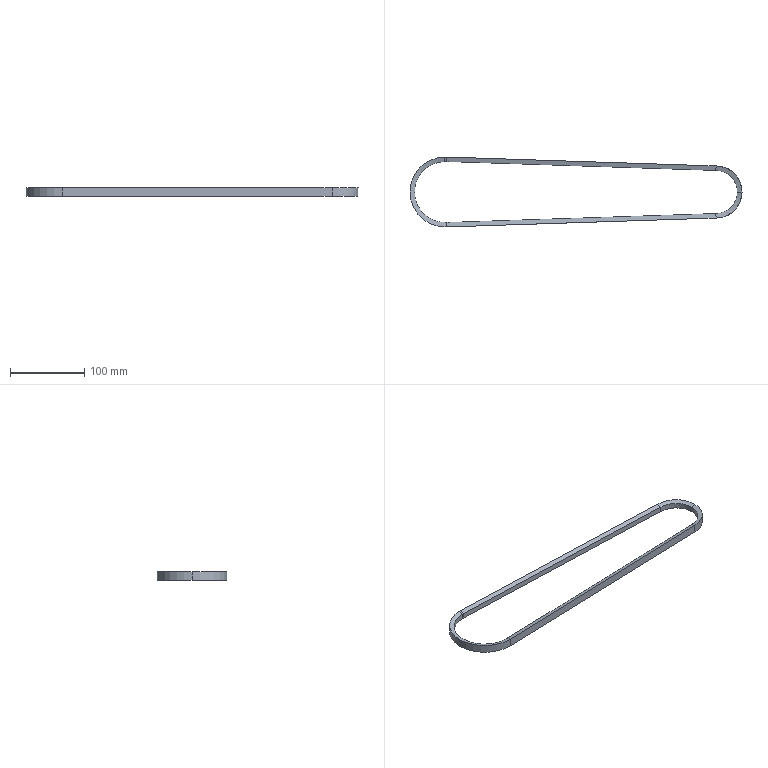Part | STEP file | Short V-belt | 1 solid | 24 faces | box 446 x 94 x 11 mm | volume 53257 mm3 | cone 8 | cylinder 8 | plane 8 | commonest cylinder face diameters 82 x3 94 x3 58 x1 70 x1
STEP:
#1=CARTESIAN_POINT('',(364.,29.,3.666));
#2=VERTEX_POINT('',#1);
#3=CARTESIAN_POINT('',(393.,0.,3.666));
#4=VERTEX_POINT('',#3);
#5=CARTESIAN_POINT('',(364.,0.,3.666));
#6=DIRECTION('',(0.,0.,-1.));
#7=DIRECTION('',(0.,1.,0.));
#8=AXIS2_PLACEMENT_3D('',#5,#6,#7);
#9=CIRCLE('',#8,29.);
#10=EDGE_CURVE('',#2,#4,#9,.T.);
#11=ORIENTED_EDGE('',*,*,#10,.T.);
#12=CARTESIAN_POINT('',(399.,0.,5.5));
#13=VERTEX_POINT('',#12);
#14=CARTESIAN_POINT('',(399.,0.,5.5));
#15=DIRECTION('',(0.9563,0.,0.2924));
#16=VECTOR('',#15,1000.);
#17=LINE('',#14,#16);
#18=EDGE_CURVE('',#4,#13,#17,.T.);
#19=ORIENTED_EDGE('',*,*,#18,.T.);
#20=CARTESIAN_POINT('',(364.104,35.,5.5));
#21=VERTEX_POINT('',#20);
#22=CARTESIAN_POINT('',(364.,0.,5.5));
#23=DIRECTION('',(0.,0.,-1.));
#24=DIRECTION('',(0.,1.,0.));
#25=AXIS2_PLACEMENT_3D('',#22,#23,#24);
#26=CIRCLE('',#25,35.);
#27=EDGE_CURVE('',#21,#13,#26,.T.);
#28=ORIENTED_EDGE('',*,*,#27,.F.);
#29=CARTESIAN_POINT('',(364.,29.,3.666));
#30=CARTESIAN_POINT('',(364.033,31.,4.277));
#31=CARTESIAN_POINT('',(364.068,33.,4.889));
#32=CARTESIAN_POINT('',(364.104,35.,5.5));
#33=B_SPLINE_CURVE_WITH_KNOTS('',3,(#29,#30,#31,#32),.UNSPECIFIED.,.F.,.F.,(4,4),(0.000000209,0.006275),.UNSPECIFIED.);
#34=EDGE_CURVE('',#2,#21,#33,.T.);
#35=ORIENTED_EDGE('',*,*,#34,.F.);
#36=EDGE_LOOP('',(#11,#19,#28,#35));
#37=FACE_OUTER_BOUND('',#36,.T.);
#38=CARTESIAN_POINT('',(364.,0.,5.5));
#39=DIRECTION('',(0.,0.,1.));
#40=DIRECTION('',(1.,0.,0.));
#41=AXIS2_PLACEMENT_3D('',#38,#39,#40);
#42=CONICAL_SURFACE('',#41,35.,1.274);
#43=ADVANCED_FACE('',(#37),#42,.F.);
#44=CARTESIAN_POINT('',(1.551,-46.974,5.5));
#45=VERTEX_POINT('',#44);
#46=CARTESIAN_POINT('',(-47.,0.,5.5));
#47=VERTEX_POINT('',#46);
#48=CARTESIAN_POINT('',(0.,0.,5.5));
#49=DIRECTION('',(0.,0.,-1.));
#50=DIRECTION('',(0.03301,-0.9995,0.));
#51=AXIS2_PLACEMENT_3D('',#48,#49,#50);
#52=CIRCLE('',#51,47.);
#53=EDGE_CURVE('',#45,#47,#52,.T.);
#54=ORIENTED_EDGE('',*,*,#53,.T.);
#55=CARTESIAN_POINT('',(-47.,0.,-5.5));
#56=VERTEX_POINT('',#55);
#57=CARTESIAN_POINT('',(-47.,0.,0.));
#58=DIRECTION('',(0.,0.,-1.));
#59=VECTOR('',#58,1000.);
#60=LINE('',#57,#59);
#61=EDGE_CURVE('',#47,#56,#60,.T.);
#62=ORIENTED_EDGE('',*,*,#61,.T.);
#63=CARTESIAN_POINT('',(1.551,-46.974,-5.5));
#64=VERTEX_POINT('',#63);
#65=CARTESIAN_POINT('',(0.,0.,-5.5));
#66=DIRECTION('',(0.,0.,-1.));
#67=DIRECTION('',(0.03301,-0.9995,0.));
#68=AXIS2_PLACEMENT_3D('',#65,#66,#67);
#69=CIRCLE('',#68,47.);
#70=EDGE_CURVE('',#64,#56,#69,.T.);
#71=ORIENTED_EDGE('',*,*,#70,.F.);
#72=CARTESIAN_POINT('',(1.551,-46.974,5.5));
#73=DIRECTION('',(0.,0.,1.));
#74=VECTOR('',#73,1000.);
#75=LINE('',#72,#74);
#76=EDGE_CURVE('',#64,#45,#75,.T.);
#77=ORIENTED_EDGE('',*,*,#76,.T.);
#78=EDGE_LOOP('',(#54,#62,#71,#77));
#79=FACE_OUTER_BOUND('',#78,.T.);
#80=CARTESIAN_POINT('',(0.,0.,0.));
#81=DIRECTION('',(0.,0.,-1.));
#82=DIRECTION('',(-1.,0.,0.));
#83=AXIS2_PLACEMENT_3D('',#80,#81,#82);
#84=CYLINDRICAL_SURFACE('',#83,47.);
#85=ADVANCED_FACE('',(#79),#84,.T.);
#86=CARTESIAN_POINT('',(-41.,0.,-3.666));
#87=VERTEX_POINT('',#86);
#88=CARTESIAN_POINT('',(0.,41.,-3.666));
#89=VERTEX_POINT('',#88);
#90=CARTESIAN_POINT('',(0.,0.,-3.666));
#91=DIRECTION('',(0.,0.,-1.));
#92=DIRECTION('',(0.03301,-0.9995,0.));
#93=AXIS2_PLACEMENT_3D('',#90,#91,#92);
#94=CIRCLE('',#93,41.);
#95=EDGE_CURVE('',#87,#89,#94,.T.);
#96=ORIENTED_EDGE('',*,*,#95,.F.);
#97=CARTESIAN_POINT('',(-41.,0.,-3.666));
#98=DIRECTION('',(-0.9563,0.,-0.2924));
#99=VECTOR('',#98,1000.);
#100=LINE('',#97,#99);
#101=EDGE_CURVE('',#87,#56,#100,.T.);
#102=ORIENTED_EDGE('',*,*,#101,.T.);
#103=CARTESIAN_POINT('',(0.,47.,-5.5));
#104=VERTEX_POINT('',#103);
#105=CARTESIAN_POINT('',(0.,0.,-5.5));
#106=DIRECTION('',(0.,0.,-1.));
#107=DIRECTION('',(0.03301,-0.9995,0.));
#108=AXIS2_PLACEMENT_3D('',#105,#106,#107);
#109=CIRCLE('',#108,47.);
#110=EDGE_CURVE('',#56,#104,#109,.T.);
#111=ORIENTED_EDGE('',*,*,#110,.T.);
#112=CARTESIAN_POINT('',(0.,47.,-5.5));
#113=DIRECTION('',(0.,0.9563,-0.2924));
#114=VECTOR('',#113,1000.);
#115=LINE('',#112,#114);
#116=EDGE_CURVE('',#89,#104,#115,.T.);
#117=ORIENTED_EDGE('',*,*,#116,.F.);
#118=EDGE_LOOP('',(#96,#102,#111,#117));
#119=FACE_OUTER_BOUND('',#118,.T.);
#120=CARTESIAN_POINT('',(0.,0.,-3.666));
#121=DIRECTION('',(0.,0.,-1.));
#122=DIRECTION('',(-1.,0.,0.));
#123=AXIS2_PLACEMENT_3D('',#120,#121,#122);
#124=CONICAL_SURFACE('',#123,41.,1.274);
#125=ADVANCED_FACE('',(#119),#124,.F.);
#126=CARTESIAN_POINT('',(-41.,0.,3.666));
#127=VERTEX_POINT('',#126);
#128=CARTESIAN_POINT('',(0.,41.,3.666));
#129=VERTEX_POINT('',#128);
#130=CARTESIAN_POINT('',(0.,0.,3.666));
#131=DIRECTION('',(0.,0.,-1.));
#132=DIRECTION('',(0.03301,-0.9995,0.));
#133=AXIS2_PLACEMENT_3D('',#130,#131,#132);
#134=CIRCLE('',#133,41.);
#135=EDGE_CURVE('',#127,#129,#134,.T.);
#136=ORIENTED_EDGE('',*,*,#135,.F.);
#137=CARTESIAN_POINT('',(-41.,0.,0.));
#138=DIRECTION('',(0.,0.,-1.));
#139=VECTOR('',#138,1000.);
#140=LINE('',#137,#139);
#141=EDGE_CURVE('',#127,#87,#140,.T.);
#142=ORIENTED_EDGE('',*,*,#141,.T.);
#143=ORIENTED_EDGE('',*,*,#95,.T.);
#144=CARTESIAN_POINT('',(0.,41.,-3.666));
#145=DIRECTION('',(0.,0.,-1.));
#146=VECTOR('',#145,1000.);
#147=LINE('',#144,#146);
#148=EDGE_CURVE('',#129,#89,#147,.T.);
#149=ORIENTED_EDGE('',*,*,#148,.F.);
#150=EDGE_LOOP('',(#136,#142,#143,#149));
#151=FACE_OUTER_BOUND('',#150,.T.);
#152=CARTESIAN_POINT('',(0.,0.,0.));
#153=DIRECTION('',(0.,0.,-1.));
#154=DIRECTION('',(-1.,0.,0.));
#155=AXIS2_PLACEMENT_3D('',#152,#153,#154);
#156=CYLINDRICAL_SURFACE('',#155,41.);
#157=ADVANCED_FACE('',(#151),#156,.F.);
#158=ORIENTED_EDGE('',*,*,#18,.F.);
#159=CARTESIAN_POINT('',(364.,-29.,3.666));
#160=VERTEX_POINT('',#159);
#161=CARTESIAN_POINT('',(364.,0.,3.666));
#162=DIRECTION('',(0.,0.,-1.));
#163=DIRECTION('',(0.,1.,0.));
#164=AXIS2_PLACEMENT_3D('',#161,#162,#163);
#165=CIRCLE('',#164,29.);
#166=EDGE_CURVE('',#4,#160,#165,.T.);
#167=ORIENTED_EDGE('',*,*,#166,.T.);
#168=CARTESIAN_POINT('',(364.104,-35.,5.5));
#169=VERTEX_POINT('',#168);
#170=CARTESIAN_POINT('',(364.,-29.,3.666));
#171=CARTESIAN_POINT('',(364.033,-31.,4.277));
#172=CARTESIAN_POINT('',(364.068,-33.,4.889));
#173=CARTESIAN_POINT('',(364.104,-35.,5.5));
#174=B_SPLINE_CURVE_WITH_KNOTS('',3,(#170,#171,#172,#173),.UNSPECIFIED.,.F.,.F.,(4,4),(0.000000209,0.006275),.UNSPECIFIED.);
#175=EDGE_CURVE('',#160,#169,#174,.T.);
#176=ORIENTED_EDGE('',*,*,#175,.T.);
#177=CARTESIAN_POINT('',(364.,0.,5.5));
#178=DIRECTION('',(0.,0.,-1.));
#179=DIRECTION('',(0.,1.,0.));
#180=AXIS2_PLACEMENT_3D('',#177,#178,#179);
#181=CIRCLE('',#180,35.);
#182=EDGE_CURVE('',#13,#169,#181,.T.);
#183=ORIENTED_EDGE('',*,*,#182,.F.);
#184=EDGE_LOOP('',(#158,#167,#176,#183));
#185=FACE_OUTER_BOUND('',#184,.T.);
#186=CARTESIAN_POINT('',(364.,0.,5.5));
#187=DIRECTION('',(0.,0.,1.));
#188=DIRECTION('',(1.,0.,0.));
#189=AXIS2_PLACEMENT_3D('',#186,#187,#188);
#190=CONICAL_SURFACE('',#189,35.,1.274);
#191=ADVANCED_FACE('',(#185),#190,.F.);
#192=CARTESIAN_POINT('',(364.104,35.,-5.5));
#193=VERTEX_POINT('',#192);
#194=CARTESIAN_POINT('',(364.,29.,-3.666));
#195=VERTEX_POINT('',#194);
#196=CARTESIAN_POINT('',(364.104,35.,-5.5));
#197=CARTESIAN_POINT('',(364.068,33.,-4.889));
#198=CARTESIAN_POINT('',(364.033,31.,-4.277));
#199=CARTESIAN_POINT('',(364.,29.,-3.666));
#200=B_SPLINE_CURVE_WITH_KNOTS('',3,(#196,#197,#198,#199),.UNSPECIFIED.,.F.,.F.,(4,4),(0.00000037,0.006275),.UNSPECIFIED.);
#201=EDGE_CURVE('',#193,#195,#200,.T.);
#202=ORIENTED_EDGE('',*,*,#201,.F.);
#203=CARTESIAN_POINT('',(364.104,-35.,-5.5));
#204=VERTEX_POINT('',#203);
#205=CARTESIAN_POINT('',(364.,0.,-5.5));
#206=DIRECTION('',(0.,0.,-1.));
#207=DIRECTION('',(0.,1.,0.));
#208=AXIS2_PLACEMENT_3D('',#205,#206,#207);
#209=CIRCLE('',#208,35.);
#210=EDGE_CURVE('',#193,#204,#209,.T.);
#211=ORIENTED_EDGE('',*,*,#210,.T.);
#212=CARTESIAN_POINT('',(364.,-29.,-3.666));
#213=VERTEX_POINT('',#212);
#214=CARTESIAN_POINT('',(364.104,-35.,-5.5));
#215=CARTESIAN_POINT('',(364.068,-33.,-4.889));
#216=CARTESIAN_POINT('',(364.033,-31.,-4.277));
#217=CARTESIAN_POINT('',(364.,-29.,-3.666));
#218=B_SPLINE_CURVE_WITH_KNOTS('',3,(#214,#215,#216,#217),.UNSPECIFIED.,.F.,.F.,(4,4),(0.00000037,0.006275),.UNSPECIFIED.);
#219=EDGE_CURVE('',#204,#213,#218,.T.);
#220=ORIENTED_EDGE('',*,*,#219,.T.);
#221=CARTESIAN_POINT('',(364.,0.,-3.666));
#222=DIRECTION('',(0.,0.,-1.));
#223=DIRECTION('',(0.,1.,0.));
#224=AXIS2_PLACEMENT_3D('',#221,#222,#223);
#225=CIRCLE('',#224,29.);
#226=EDGE_CURVE('',#195,#213,#225,.T.);
#227=ORIENTED_EDGE('',*,*,#226,.F.);
#228=EDGE_LOOP('',(#202,#211,#220,#227));
#229=FACE_OUTER_BOUND('',#228,.T.);
#230=CARTESIAN_POINT('',(364.,0.,-3.666));
#231=DIRECTION('',(0.,0.,-1.));
#232=DIRECTION('',(-1.,0.,0.));
#233=AXIS2_PLACEMENT_3D('',#230,#231,#232);
#234=CONICAL_SURFACE('',#233,29.,1.274);
#235=ADVANCED_FACE('',(#229),#234,.F.);
#236=ORIENTED_EDGE('',*,*,#210,.F.);
#237=CARTESIAN_POINT('',(364.104,35.,0.));
#238=DIRECTION('',(0.,0.,1.));
#239=VECTOR('',#238,1000.);
#240=LINE('',#237,#239);
#241=EDGE_CURVE('',#193,#21,#240,.T.);
#242=ORIENTED_EDGE('',*,*,#241,.T.);
#243=ORIENTED_EDGE('',*,*,#27,.T.);
#244=ORIENTED_EDGE('',*,*,#182,.T.);
#245=CARTESIAN_POINT('',(364.104,-35.,0.));
#246=DIRECTION('',(0.,0.,1.));
#247=VECTOR('',#246,1000.);
#248=LINE('',#245,#247);
#249=EDGE_CURVE('',#204,#169,#248,.T.);
#250=ORIENTED_EDGE('',*,*,#249,.F.);
#251=EDGE_LOOP('',(#236,#242,#243,#244,#250));
#252=FACE_OUTER_BOUND('',#251,.T.);
#253=CARTESIAN_POINT('',(364.,0.,0.));
#254=DIRECTION('',(0.,0.,-1.));
#255=DIRECTION('',(-1.,0.,0.));
#256=AXIS2_PLACEMENT_3D('',#253,#254,#255);
#257=CYLINDRICAL_SURFACE('',#256,35.);
#258=ADVANCED_FACE('',(#252),#257,.T.);
#259=ORIENTED_EDGE('',*,*,#226,.T.);
#260=CARTESIAN_POINT('',(364.,-29.,-3.666));
#261=DIRECTION('',(0.,0.,-1.));
#262=VECTOR('',#261,1000.);
#263=LINE('',#260,#262);
#264=EDGE_CURVE('',#160,#213,#263,.T.);
#265=ORIENTED_EDGE('',*,*,#264,.F.);
#266=ORIENTED_EDGE('',*,*,#166,.F.);
#267=ORIENTED_EDGE('',*,*,#10,.F.);
#268=CARTESIAN_POINT('',(364.,29.,-3.666));
#269=DIRECTION('',(0.,0.,-1.));
#270=VECTOR('',#269,1000.);
#271=LINE('',#268,#270);
#272=EDGE_CURVE('',#2,#195,#271,.T.);
#273=ORIENTED_EDGE('',*,*,#272,.T.);
#274=EDGE_LOOP('',(#259,#265,#266,#267,#273));
#275=FACE_OUTER_BOUND('',#274,.T.);
#276=CARTESIAN_POINT('',(364.,0.,0.));
#277=DIRECTION('',(0.,0.,-1.));
#278=DIRECTION('',(-1.,0.,0.));
#279=AXIS2_PLACEMENT_3D('',#276,#277,#278);
#280=CYLINDRICAL_SURFACE('',#279,29.);
#281=ADVANCED_FACE('',(#275),#280,.F.);
#282=ORIENTED_EDGE('',*,*,#175,.F.);
#283=CARTESIAN_POINT('',(1.353,-40.978,3.666));
#284=VERTEX_POINT('',#283);
#285=CARTESIAN_POINT('',(364.,-29.,3.666));
#286=DIRECTION('',(-0.9995,-0.03301,0.));
#287=VECTOR('',#286,1000.);
#288=LINE('',#285,#287);
#289=EDGE_CURVE('',#160,#284,#288,.T.);
#290=ORIENTED_EDGE('',*,*,#289,.T.);
#291=CARTESIAN_POINT('',(1.551,-46.974,5.5));
#292=DIRECTION('',(-0.03157,0.9558,-0.2924));
#293=VECTOR('',#292,1000.);
#294=LINE('',#291,#293);
#295=EDGE_CURVE('',#45,#284,#294,.T.);
#296=ORIENTED_EDGE('',*,*,#295,.F.);
#297=CARTESIAN_POINT('',(364.198,-34.997,5.5));
#298=DIRECTION('',(-0.9995,-0.03301,0.));
#299=VECTOR('',#298,1000.);
#300=LINE('',#297,#299);
#301=EDGE_CURVE('',#169,#45,#300,.T.);
#302=ORIENTED_EDGE('',*,*,#301,.F.);
#303=EDGE_LOOP('',(#282,#290,#296,#302));
#304=FACE_OUTER_BOUND('',#303,.T.);
#305=CARTESIAN_POINT('',(364.198,-34.997,5.5));
#306=DIRECTION('',(-0.009651,0.2922,0.9563));
#307=DIRECTION('',(0.,-0.9563,0.2922));
#308=AXIS2_PLACEMENT_3D('',#305,#306,#307);
#309=PLANE('',#308);
#310=ADVANCED_FACE('',(#304),#309,.T.);
#311=ORIENTED_EDGE('',*,*,#219,.F.);
#312=CARTESIAN_POINT('',(364.198,-34.997,-5.5));
#313=DIRECTION('',(-0.9995,-0.03301,0.));
#314=VECTOR('',#313,1000.);
#315=LINE('',#312,#314);
#316=EDGE_CURVE('',#204,#64,#315,.T.);
#317=ORIENTED_EDGE('',*,*,#316,.T.);
#318=CARTESIAN_POINT('',(1.353,-40.978,-3.666));
#319=VERTEX_POINT('',#318);
#320=CARTESIAN_POINT('',(1.551,-46.974,-5.5));
#321=DIRECTION('',(0.03157,-0.9558,-0.2924));
#322=VECTOR('',#321,1000.);
#323=LINE('',#320,#322);
#324=EDGE_CURVE('',#319,#64,#323,.T.);
#325=ORIENTED_EDGE('',*,*,#324,.F.);
#326=CARTESIAN_POINT('',(364.,-29.,-3.666));
#327=DIRECTION('',(-0.9995,-0.03301,0.));
#328=VECTOR('',#327,1000.);
#329=LINE('',#326,#328);
#330=EDGE_CURVE('',#213,#319,#329,.T.);
#331=ORIENTED_EDGE('',*,*,#330,.F.);
#332=EDGE_LOOP('',(#311,#317,#325,#331));
#333=FACE_OUTER_BOUND('',#332,.T.);
#334=CARTESIAN_POINT('',(364.198,-34.997,-5.5));
#335=DIRECTION('',(-0.009651,0.2922,-0.9563));
#336=DIRECTION('',(0.,0.9563,0.2922));
#337=AXIS2_PLACEMENT_3D('',#334,#335,#336);
#338=PLANE('',#337);
#339=ADVANCED_FACE('',(#333),#338,.T.);
#340=ORIENTED_EDGE('',*,*,#330,.T.);
#341=CARTESIAN_POINT('',(1.353,-40.978,-3.666));
#342=DIRECTION('',(0.,0.,-1.));
#343=VECTOR('',#342,1000.);
#344=LINE('',#341,#343);
#345=EDGE_CURVE('',#284,#319,#344,.T.);
#346=ORIENTED_EDGE('',*,*,#345,.F.);
#347=ORIENTED_EDGE('',*,*,#289,.F.);
#348=ORIENTED_EDGE('',*,*,#264,.T.);
#349=EDGE_LOOP('',(#340,#346,#347,#348));
#350=FACE_OUTER_BOUND('',#349,.T.);
#351=CARTESIAN_POINT('',(364.,-29.,-3.666));
#352=DIRECTION('',(-0.03301,0.9995,0.));
#353=DIRECTION('',(-0.9995,-0.03301,0.));
#354=AXIS2_PLACEMENT_3D('',#351,#352,#353);
#355=PLANE('',#354);
#356=ADVANCED_FACE('',(#350),#355,.T.);
#357=ORIENTED_EDGE('',*,*,#316,.F.);
#358=ORIENTED_EDGE('',*,*,#249,.T.);
#359=ORIENTED_EDGE('',*,*,#301,.T.);
#360=ORIENTED_EDGE('',*,*,#76,.F.);
#361=EDGE_LOOP('',(#357,#358,#359,#360));
#362=FACE_OUTER_BOUND('',#361,.T.);
#363=CARTESIAN_POINT('',(364.198,-34.997,5.5));
#364=DIRECTION('',(0.03301,-0.9995,0.));
#365=DIRECTION('',(0.9995,0.03301,0.));
#366=AXIS2_PLACEMENT_3D('',#363,#364,#365);
#367=PLANE('',#366);
#368=ADVANCED_FACE('',(#362),#367,.T.);
#369=CARTESIAN_POINT('',(1.353,40.978,3.666));
#370=VERTEX_POINT('',#369);
#371=CARTESIAN_POINT('',(1.353,40.978,3.666));
#372=DIRECTION('',(0.9995,-0.03301,0.));
#373=VECTOR('',#372,1000.);
#374=LINE('',#371,#373);
#375=EDGE_CURVE('',#370,#2,#374,.T.);
#376=ORIENTED_EDGE('',*,*,#375,.T.);
#377=ORIENTED_EDGE('',*,*,#34,.T.);
#378=CARTESIAN_POINT('',(1.551,46.974,5.5));
#379=VERTEX_POINT('',#378);
#380=CARTESIAN_POINT('',(1.551,46.974,5.5));
#381=DIRECTION('',(0.9995,-0.03301,0.));
#382=VECTOR('',#381,1000.);
#383=LINE('',#380,#382);
#384=EDGE_CURVE('',#379,#21,#383,.T.);
#385=ORIENTED_EDGE('',*,*,#384,.F.);
#386=CARTESIAN_POINT('',(1.551,46.974,5.5));
#387=DIRECTION('',(-0.03157,-0.9558,-0.2924));
#388=VECTOR('',#387,1000.);
#389=LINE('',#386,#388);
#390=EDGE_CURVE('',#379,#370,#389,.T.);
#391=ORIENTED_EDGE('',*,*,#390,.T.);
#392=EDGE_LOOP('',(#376,#377,#385,#391));
#393=FACE_OUTER_BOUND('',#392,.T.);
#394=CARTESIAN_POINT('',(1.551,46.974,5.5));
#395=DIRECTION('',(-0.009651,-0.2922,0.9563));
#396=DIRECTION('',(0.,-0.9563,-0.2922));
#397=AXIS2_PLACEMENT_3D('',#394,#395,#396);
#398=PLANE('',#397);
#399=ADVANCED_FACE('',(#393),#398,.T.);
#400=CARTESIAN_POINT('',(1.551,46.974,-5.5));
#401=VERTEX_POINT('',#400);
#402=CARTESIAN_POINT('',(1.551,46.974,-5.5));
#403=DIRECTION('',(0.9995,-0.03301,0.));
#404=VECTOR('',#403,1000.);
#405=LINE('',#402,#404);
#406=EDGE_CURVE('',#401,#193,#405,.T.);
#407=ORIENTED_EDGE('',*,*,#406,.T.);
#408=ORIENTED_EDGE('',*,*,#201,.T.);
#409=CARTESIAN_POINT('',(1.353,40.978,-3.666));
#410=VERTEX_POINT('',#409);
#411=CARTESIAN_POINT('',(1.353,40.978,-3.666));
#412=DIRECTION('',(0.9995,-0.03301,0.));
#413=VECTOR('',#412,1000.);
#414=LINE('',#411,#413);
#415=EDGE_CURVE('',#410,#195,#414,.T.);
#416=ORIENTED_EDGE('',*,*,#415,.F.);
#417=CARTESIAN_POINT('',(1.551,46.974,-5.5));
#418=DIRECTION('',(0.03157,0.9558,-0.2924));
#419=VECTOR('',#418,1000.);
#420=LINE('',#417,#419);
#421=EDGE_CURVE('',#410,#401,#420,.T.);
#422=ORIENTED_EDGE('',*,*,#421,.T.);
#423=EDGE_LOOP('',(#407,#408,#416,#422));
#424=FACE_OUTER_BOUND('',#423,.T.);
#425=CARTESIAN_POINT('',(1.551,46.974,-5.5));
#426=DIRECTION('',(-0.009651,-0.2922,-0.9563));
#427=DIRECTION('',(0.,0.9563,-0.2922));
#428=AXIS2_PLACEMENT_3D('',#425,#426,#427);
#429=PLANE('',#428);
#430=ADVANCED_FACE('',(#424),#429,.T.);
#431=ORIENTED_EDGE('',*,*,#241,.F.);
#432=ORIENTED_EDGE('',*,*,#406,.F.);
#433=CARTESIAN_POINT('',(1.551,46.974,5.5));
#434=DIRECTION('',(0.,0.,1.));
#435=VECTOR('',#434,1000.);
#436=LINE('',#433,#435);
#437=EDGE_CURVE('',#401,#379,#436,.T.);
#438=ORIENTED_EDGE('',*,*,#437,.T.);
#439=ORIENTED_EDGE('',*,*,#384,.T.);
#440=EDGE_LOOP('',(#431,#432,#438,#439));
#441=FACE_OUTER_BOUND('',#440,.T.);
#442=CARTESIAN_POINT('',(1.551,46.974,5.5));
#443=DIRECTION('',(0.03301,0.9995,0.));
#444=DIRECTION('',(-0.9995,0.03301,0.));
#445=AXIS2_PLACEMENT_3D('',#442,#443,#444);
#446=PLANE('',#445);
#447=ADVANCED_FACE('',(#441),#446,.T.);
#448=ORIENTED_EDGE('',*,*,#415,.T.);
#449=ORIENTED_EDGE('',*,*,#272,.F.);
#450=ORIENTED_EDGE('',*,*,#375,.F.);
#451=CARTESIAN_POINT('',(1.353,40.978,-3.666));
#452=DIRECTION('',(0.,0.,-1.));
#453=VECTOR('',#452,1000.);
#454=LINE('',#451,#453);
#455=EDGE_CURVE('',#370,#410,#454,.T.);
#456=ORIENTED_EDGE('',*,*,#455,.T.);
#457=EDGE_LOOP('',(#448,#449,#450,#456));
#458=FACE_OUTER_BOUND('',#457,.T.);
#459=CARTESIAN_POINT('',(1.353,40.978,-3.666));
#460=DIRECTION('',(-0.03301,-0.9995,0.));
#461=DIRECTION('',(0.9995,-0.03301,0.));
#462=AXIS2_PLACEMENT_3D('',#459,#460,#461);
#463=PLANE('',#462);
#464=ADVANCED_FACE('',(#458),#463,.T.);
#465=ORIENTED_EDGE('',*,*,#437,.F.);
#466=CARTESIAN_POINT('',(0.,0.,-5.5));
#467=DIRECTION('',(0.,0.,-1.));
#468=DIRECTION('',(0.,1.,0.));
#469=AXIS2_PLACEMENT_3D('',#466,#467,#468);
#470=CIRCLE('',#469,47.);
#471=EDGE_CURVE('',#104,#401,#470,.T.);
#472=ORIENTED_EDGE('',*,*,#471,.F.);
#473=CARTESIAN_POINT('',(0.,47.,5.5));
#474=VERTEX_POINT('',#473);
#475=CARTESIAN_POINT('',(0.,47.,5.5));
#476=DIRECTION('',(0.,0.,1.));
#477=VECTOR('',#476,1000.);
#478=LINE('',#475,#477);
#479=EDGE_CURVE('',#104,#474,#478,.T.);
#480=ORIENTED_EDGE('',*,*,#479,.T.);
#481=CARTESIAN_POINT('',(0.,0.,5.5));
#482=DIRECTION('',(0.,0.,-1.));
#483=DIRECTION('',(0.,1.,0.));
#484=AXIS2_PLACEMENT_3D('',#481,#482,#483);
#485=CIRCLE('',#484,47.);
#486=EDGE_CURVE('',#474,#379,#485,.T.);
#487=ORIENTED_EDGE('',*,*,#486,.T.);
#488=EDGE_LOOP('',(#465,#472,#480,#487));
#489=FACE_OUTER_BOUND('',#488,.T.);
#490=CARTESIAN_POINT('',(0.,0.,0.));
#491=DIRECTION('',(0.,0.,-1.));
#492=DIRECTION('',(-1.,0.,0.));
#493=AXIS2_PLACEMENT_3D('',#490,#491,#492);
#494=CYLINDRICAL_SURFACE('',#493,47.);
#495=ADVANCED_FACE('',(#489),#494,.T.);
#496=ORIENTED_EDGE('',*,*,#471,.T.);
#497=ORIENTED_EDGE('',*,*,#421,.F.);
#498=CARTESIAN_POINT('',(0.,0.,-3.666));
#499=DIRECTION('',(0.,0.,-1.));
#500=DIRECTION('',(0.,1.,0.));
#501=AXIS2_PLACEMENT_3D('',#498,#499,#500);
#502=CIRCLE('',#501,41.);
#503=EDGE_CURVE('',#89,#410,#502,.T.);
#504=ORIENTED_EDGE('',*,*,#503,.F.);
#505=ORIENTED_EDGE('',*,*,#116,.T.);
#506=EDGE_LOOP('',(#496,#497,#504,#505));
#507=FACE_OUTER_BOUND('',#506,.T.);
#508=CARTESIAN_POINT('',(0.,0.,-3.666));
#509=DIRECTION('',(0.,0.,-1.));
#510=DIRECTION('',(-1.,0.,0.));
#511=AXIS2_PLACEMENT_3D('',#508,#509,#510);
#512=CONICAL_SURFACE('',#511,41.,1.274);
#513=ADVANCED_FACE('',(#507),#512,.F.);
#514=ORIENTED_EDGE('',*,*,#503,.T.);
#515=ORIENTED_EDGE('',*,*,#455,.F.);
#516=CARTESIAN_POINT('',(0.,0.,3.666));
#517=DIRECTION('',(0.,0.,-1.));
#518=DIRECTION('',(0.,1.,0.));
#519=AXIS2_PLACEMENT_3D('',#516,#517,#518);
#520=CIRCLE('',#519,41.);
#521=EDGE_CURVE('',#129,#370,#520,.T.);
#522=ORIENTED_EDGE('',*,*,#521,.F.);
#523=ORIENTED_EDGE('',*,*,#148,.T.);
#524=EDGE_LOOP('',(#514,#515,#522,#523));
#525=FACE_OUTER_BOUND('',#524,.T.);
#526=CARTESIAN_POINT('',(0.,0.,0.));
#527=DIRECTION('',(0.,0.,-1.));
#528=DIRECTION('',(-1.,0.,0.));
#529=AXIS2_PLACEMENT_3D('',#526,#527,#528);
#530=CYLINDRICAL_SURFACE('',#529,41.);
#531=ADVANCED_FACE('',(#525),#530,.F.);
#532=ORIENTED_EDGE('',*,*,#521,.T.);
#533=ORIENTED_EDGE('',*,*,#390,.F.);
#534=ORIENTED_EDGE('',*,*,#486,.F.);
#535=CARTESIAN_POINT('',(0.,47.,5.5));
#536=DIRECTION('',(0.,-0.9563,-0.2924));
#537=VECTOR('',#536,1000.);
#538=LINE('',#535,#537);
#539=EDGE_CURVE('',#474,#129,#538,.T.);
#540=ORIENTED_EDGE('',*,*,#539,.T.);
#541=EDGE_LOOP('',(#532,#533,#534,#540));
#542=FACE_OUTER_BOUND('',#541,.T.);
#543=CARTESIAN_POINT('',(0.,0.,5.5));
#544=DIRECTION('',(0.,0.,1.));
#545=DIRECTION('',(1.,0.,0.));
#546=AXIS2_PLACEMENT_3D('',#543,#544,#545);
#547=CONICAL_SURFACE('',#546,47.,1.274);
#548=ADVANCED_FACE('',(#542),#547,.F.);
#549=ORIENTED_EDGE('',*,*,#61,.F.);
#550=CARTESIAN_POINT('',(0.,0.,5.5));
#551=DIRECTION('',(0.,0.,-1.));
#552=DIRECTION('',(0.03301,-0.9995,0.));
#553=AXIS2_PLACEMENT_3D('',#550,#551,#552);
#554=CIRCLE('',#553,47.);
#555=EDGE_CURVE('',#47,#474,#554,.T.);
#556=ORIENTED_EDGE('',*,*,#555,.T.);
#557=ORIENTED_EDGE('',*,*,#479,.F.);
#558=ORIENTED_EDGE('',*,*,#110,.F.);
#559=EDGE_LOOP('',(#549,#556,#557,#558));
#560=FACE_OUTER_BOUND('',#559,.T.);
#561=CARTESIAN_POINT('',(0.,0.,0.));
#562=DIRECTION('',(0.,0.,-1.));
#563=DIRECTION('',(-1.,0.,0.));
#564=AXIS2_PLACEMENT_3D('',#561,#562,#563);
#565=CYLINDRICAL_SURFACE('',#564,47.);
#566=ADVANCED_FACE('',(#560),#565,.T.);
#567=ORIENTED_EDGE('',*,*,#101,.F.);
#568=CARTESIAN_POINT('',(0.,0.,-3.666));
#569=DIRECTION('',(0.,0.,-1.));
#570=DIRECTION('',(0.03301,-0.9995,0.));
#571=AXIS2_PLACEMENT_3D('',#568,#569,#570);
#572=CIRCLE('',#571,41.);
#573=EDGE_CURVE('',#319,#87,#572,.T.);
#574=ORIENTED_EDGE('',*,*,#573,.F.);
#575=ORIENTED_EDGE('',*,*,#324,.T.);
#576=ORIENTED_EDGE('',*,*,#70,.T.);
#577=EDGE_LOOP('',(#567,#574,#575,#576));
#578=FACE_OUTER_BOUND('',#577,.T.);
#579=CARTESIAN_POINT('',(0.,0.,-3.666));
#580=DIRECTION('',(0.,0.,-1.));
#581=DIRECTION('',(-1.,0.,0.));
#582=AXIS2_PLACEMENT_3D('',#579,#580,#581);
#583=CONICAL_SURFACE('',#582,41.,1.274);
#584=ADVANCED_FACE('',(#578),#583,.F.);
#585=ORIENTED_EDGE('',*,*,#141,.F.);
#586=CARTESIAN_POINT('',(0.,0.,3.666));
#587=DIRECTION('',(0.,0.,-1.));
#588=DIRECTION('',(0.03301,-0.9995,0.));
#589=AXIS2_PLACEMENT_3D('',#586,#587,#588);
#590=CIRCLE('',#589,41.);
#591=EDGE_CURVE('',#284,#127,#590,.T.);
#592=ORIENTED_EDGE('',*,*,#591,.F.);
#593=ORIENTED_EDGE('',*,*,#345,.T.);
#594=ORIENTED_EDGE('',*,*,#573,.T.);
#595=EDGE_LOOP('',(#585,#592,#593,#594));
#596=FACE_OUTER_BOUND('',#595,.T.);
#597=CARTESIAN_POINT('',(0.,0.,0.));
#598=DIRECTION('',(0.,0.,-1.));
#599=DIRECTION('',(-1.,0.,0.));
#600=AXIS2_PLACEMENT_3D('',#597,#598,#599);
#601=CYLINDRICAL_SURFACE('',#600,41.);
#602=ADVANCED_FACE('',(#596),#601,.F.);
#603=ORIENTED_EDGE('',*,*,#591,.T.);
#604=ORIENTED_EDGE('',*,*,#135,.T.);
#605=ORIENTED_EDGE('',*,*,#539,.F.);
#606=ORIENTED_EDGE('',*,*,#555,.F.);
#607=ORIENTED_EDGE('',*,*,#53,.F.);
#608=ORIENTED_EDGE('',*,*,#295,.T.);
#609=EDGE_LOOP('',(#603,#604,#605,#606,#607,#608));
#610=FACE_OUTER_BOUND('',#609,.T.);
#611=CARTESIAN_POINT('',(0.,0.,5.5));
#612=DIRECTION('',(0.,0.,1.));
#613=DIRECTION('',(1.,0.,0.));
#614=AXIS2_PLACEMENT_3D('',#611,#612,#613);
#615=CONICAL_SURFACE('',#614,47.,1.274);
#616=ADVANCED_FACE('',(#610),#615,.F.);
#617=CLOSED_SHELL('',(#43,#85,#125,#157,#191,#235,#258,#281,#310,#339,#356,#368,#399,#430,#447,#464,#495,#513,#531,#548,#566,#584,#602,#616));
#618=MANIFOLD_SOLID_BREP('',#617);
#619=CARTESIAN_POINT('',(0.,0.,0.));
#620=DIRECTION('',(0.,0.,1.));
#621=DIRECTION('',(1.,0.,0.));
#622=AXIS2_PLACEMENT_3D('',#619,#620,#621);
#623=(LENGTH_UNIT()NAMED_UNIT(*)SI_UNIT(.MILLI.,.METRE.));
#624=UNCERTAINTY_MEASURE_WITH_UNIT(LENGTH_MEASURE(0.00001),#623,'','');
#625=(NAMED_UNIT(*)PLANE_ANGLE_UNIT()SI_UNIT($,.RADIAN.));
#626=(NAMED_UNIT(*)SI_UNIT($,.STERADIAN.)SOLID_ANGLE_UNIT());
#627=(GEOMETRIC_REPRESENTATION_CONTEXT(3)GLOBAL_UNCERTAINTY_ASSIGNED_CONTEXT((#624))GLOBAL_UNIT_ASSIGNED_CONTEXT((#623,#625,#626))REPRESENTATION_CONTEXT('',''));
#628=ADVANCED_BREP_SHAPE_REPRESENTATION('',(#618,#622),#627);